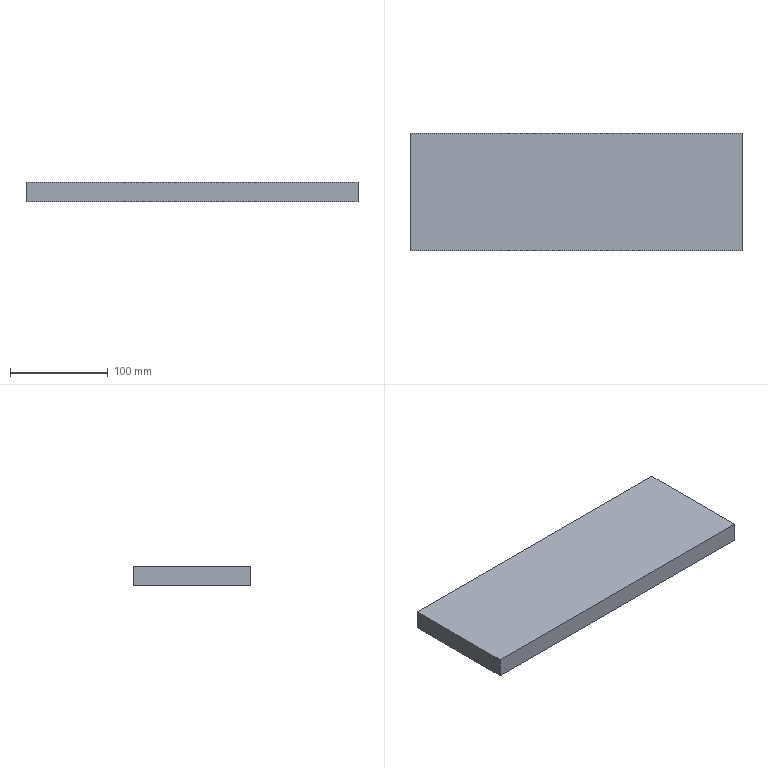Part | SolidWorks | features Extrusion 1 | 1 solid | 6 faces | box 340 x 120 x 20 mm | volume 816000 mm3 | plane 6
STEP:
#1=CARTESIAN_POINT('',(0.,120.,0.));
#2=VERTEX_POINT('',#1);
#3=CARTESIAN_POINT('',(0.,0.,0.));
#4=VERTEX_POINT('',#3);
#5=CARTESIAN_POINT('',(0.,0.,0.));
#6=DIRECTION('',(0.,-1.,0.));
#7=VECTOR('',#6,1000.);
#8=LINE('',#5,#7);
#9=EDGE_CURVE('',#2,#4,#8,.T.);
#10=ORIENTED_EDGE('',*,*,#9,.T.);
#11=CARTESIAN_POINT('',(0.,0.,20.));
#12=VERTEX_POINT('',#11);
#13=CARTESIAN_POINT('',(0.,0.,20.));
#14=DIRECTION('',(0.,0.,-1.));
#15=VECTOR('',#14,1000.);
#16=LINE('',#13,#15);
#17=EDGE_CURVE('',#12,#4,#16,.T.);
#18=ORIENTED_EDGE('',*,*,#17,.F.);
#19=CARTESIAN_POINT('',(0.,120.,20.));
#20=VERTEX_POINT('',#19);
#21=CARTESIAN_POINT('',(0.,0.,20.));
#22=DIRECTION('',(0.,-1.,0.));
#23=VECTOR('',#22,1000.);
#24=LINE('',#21,#23);
#25=EDGE_CURVE('',#20,#12,#24,.T.);
#26=ORIENTED_EDGE('',*,*,#25,.F.);
#27=CARTESIAN_POINT('',(0.,120.,20.));
#28=DIRECTION('',(0.,0.,-1.));
#29=VECTOR('',#28,1000.);
#30=LINE('',#27,#29);
#31=EDGE_CURVE('',#20,#2,#30,.T.);
#32=ORIENTED_EDGE('',*,*,#31,.T.);
#33=EDGE_LOOP('',(#10,#18,#26,#32));
#34=FACE_OUTER_BOUND('',#33,.T.);
#35=CARTESIAN_POINT('',(0.,0.,20.));
#36=DIRECTION('',(1.,0.,0.));
#37=DIRECTION('',(0.,0.,-1.));
#38=AXIS2_PLACEMENT_3D('',#35,#36,#37);
#39=PLANE('',#38);
#40=ADVANCED_FACE('',(#34),#39,.F.);
#41=CARTESIAN_POINT('',(340.,0.,0.));
#42=VERTEX_POINT('',#41);
#43=CARTESIAN_POINT('',(0.,0.,0.));
#44=DIRECTION('',(1.,0.,0.));
#45=VECTOR('',#44,1000.);
#46=LINE('',#43,#45);
#47=EDGE_CURVE('',#4,#42,#46,.T.);
#48=ORIENTED_EDGE('',*,*,#47,.T.);
#49=CARTESIAN_POINT('',(340.,0.,20.));
#50=VERTEX_POINT('',#49);
#51=CARTESIAN_POINT('',(340.,0.,20.));
#52=DIRECTION('',(0.,0.,-1.));
#53=VECTOR('',#52,1000.);
#54=LINE('',#51,#53);
#55=EDGE_CURVE('',#50,#42,#54,.T.);
#56=ORIENTED_EDGE('',*,*,#55,.F.);
#57=CARTESIAN_POINT('',(0.,0.,20.));
#58=DIRECTION('',(1.,0.,0.));
#59=VECTOR('',#58,1000.);
#60=LINE('',#57,#59);
#61=EDGE_CURVE('',#12,#50,#60,.T.);
#62=ORIENTED_EDGE('',*,*,#61,.F.);
#63=ORIENTED_EDGE('',*,*,#17,.T.);
#64=EDGE_LOOP('',(#48,#56,#62,#63));
#65=FACE_OUTER_BOUND('',#64,.T.);
#66=CARTESIAN_POINT('',(0.,0.,20.));
#67=DIRECTION('',(0.,1.,0.));
#68=DIRECTION('',(0.,0.,1.));
#69=AXIS2_PLACEMENT_3D('',#66,#67,#68);
#70=PLANE('',#69);
#71=ADVANCED_FACE('',(#65),#70,.F.);
#72=CARTESIAN_POINT('',(340.,120.,0.));
#73=VERTEX_POINT('',#72);
#74=CARTESIAN_POINT('',(340.,0.,0.));
#75=DIRECTION('',(0.,1.,0.));
#76=VECTOR('',#75,1000.);
#77=LINE('',#74,#76);
#78=EDGE_CURVE('',#42,#73,#77,.T.);
#79=ORIENTED_EDGE('',*,*,#78,.T.);
#80=CARTESIAN_POINT('',(340.,120.,20.));
#81=VERTEX_POINT('',#80);
#82=CARTESIAN_POINT('',(340.,120.,20.));
#83=DIRECTION('',(0.,0.,-1.));
#84=VECTOR('',#83,1000.);
#85=LINE('',#82,#84);
#86=EDGE_CURVE('',#81,#73,#85,.T.);
#87=ORIENTED_EDGE('',*,*,#86,.F.);
#88=CARTESIAN_POINT('',(340.,0.,20.));
#89=DIRECTION('',(0.,1.,0.));
#90=VECTOR('',#89,1000.);
#91=LINE('',#88,#90);
#92=EDGE_CURVE('',#50,#81,#91,.T.);
#93=ORIENTED_EDGE('',*,*,#92,.F.);
#94=ORIENTED_EDGE('',*,*,#55,.T.);
#95=EDGE_LOOP('',(#79,#87,#93,#94));
#96=FACE_OUTER_BOUND('',#95,.T.);
#97=CARTESIAN_POINT('',(340.,0.,20.));
#98=DIRECTION('',(-1.,0.,0.));
#99=DIRECTION('',(0.,0.,1.));
#100=AXIS2_PLACEMENT_3D('',#97,#98,#99);
#101=PLANE('',#100);
#102=ADVANCED_FACE('',(#96),#101,.F.);
#103=CARTESIAN_POINT('',(0.,120.,0.));
#104=DIRECTION('',(-1.,0.,0.));
#105=VECTOR('',#104,1000.);
#106=LINE('',#103,#105);
#107=EDGE_CURVE('',#73,#2,#106,.T.);
#108=ORIENTED_EDGE('',*,*,#107,.T.);
#109=ORIENTED_EDGE('',*,*,#31,.F.);
#110=CARTESIAN_POINT('',(0.,120.,20.));
#111=DIRECTION('',(-1.,0.,0.));
#112=VECTOR('',#111,1000.);
#113=LINE('',#110,#112);
#114=EDGE_CURVE('',#81,#20,#113,.T.);
#115=ORIENTED_EDGE('',*,*,#114,.F.);
#116=ORIENTED_EDGE('',*,*,#86,.T.);
#117=EDGE_LOOP('',(#108,#109,#115,#116));
#118=FACE_OUTER_BOUND('',#117,.T.);
#119=CARTESIAN_POINT('',(0.,120.,20.));
#120=DIRECTION('',(0.,-1.,0.));
#121=DIRECTION('',(0.,0.,-1.));
#122=AXIS2_PLACEMENT_3D('',#119,#120,#121);
#123=PLANE('',#122);
#124=ADVANCED_FACE('',(#118),#123,.F.);
#125=ORIENTED_EDGE('',*,*,#25,.T.);
#126=ORIENTED_EDGE('',*,*,#61,.T.);
#127=ORIENTED_EDGE('',*,*,#92,.T.);
#128=ORIENTED_EDGE('',*,*,#114,.T.);
#129=EDGE_LOOP('',(#125,#126,#127,#128));
#130=FACE_OUTER_BOUND('',#129,.T.);
#131=CARTESIAN_POINT('',(0.,0.,20.));
#132=DIRECTION('',(0.,0.,-1.));
#133=DIRECTION('',(-1.,0.,0.));
#134=AXIS2_PLACEMENT_3D('',#131,#132,#133);
#135=PLANE('',#134);
#136=ADVANCED_FACE('',(#130),#135,.F.);
#137=ORIENTED_EDGE('',*,*,#9,.F.);
#138=ORIENTED_EDGE('',*,*,#107,.F.);
#139=ORIENTED_EDGE('',*,*,#78,.F.);
#140=ORIENTED_EDGE('',*,*,#47,.F.);
#141=EDGE_LOOP('',(#137,#138,#139,#140));
#142=FACE_OUTER_BOUND('',#141,.T.);
#143=CARTESIAN_POINT('',(0.,0.,0.));
#144=DIRECTION('',(0.,0.,-1.));
#145=DIRECTION('',(-1.,0.,0.));
#146=AXIS2_PLACEMENT_3D('',#143,#144,#145);
#147=PLANE('',#146);
#148=ADVANCED_FACE('',(#142),#147,.T.);
#149=CLOSED_SHELL('',(#40,#71,#102,#124,#136,#148));
#150=MANIFOLD_SOLID_BREP('',#149);
#151=CARTESIAN_POINT('',(0.,0.,0.));
#152=DIRECTION('',(0.,0.,1.));
#153=DIRECTION('',(1.,0.,0.));
#154=AXIS2_PLACEMENT_3D('',#151,#152,#153);
#155=(LENGTH_UNIT()NAMED_UNIT(*)SI_UNIT(.MILLI.,.METRE.));
#156=UNCERTAINTY_MEASURE_WITH_UNIT(LENGTH_MEASURE(0.00001),#155,'','');
#157=(NAMED_UNIT(*)PLANE_ANGLE_UNIT()SI_UNIT($,.RADIAN.));
#158=(NAMED_UNIT(*)SI_UNIT($,.STERADIAN.)SOLID_ANGLE_UNIT());
#159=(GEOMETRIC_REPRESENTATION_CONTEXT(3)GLOBAL_UNCERTAINTY_ASSIGNED_CONTEXT((#156))GLOBAL_UNIT_ASSIGNED_CONTEXT((#155,#157,#158))REPRESENTATION_CONTEXT('',''));
#160=ADVANCED_BREP_SHAPE_REPRESENTATION('',(#150,#154),#159);